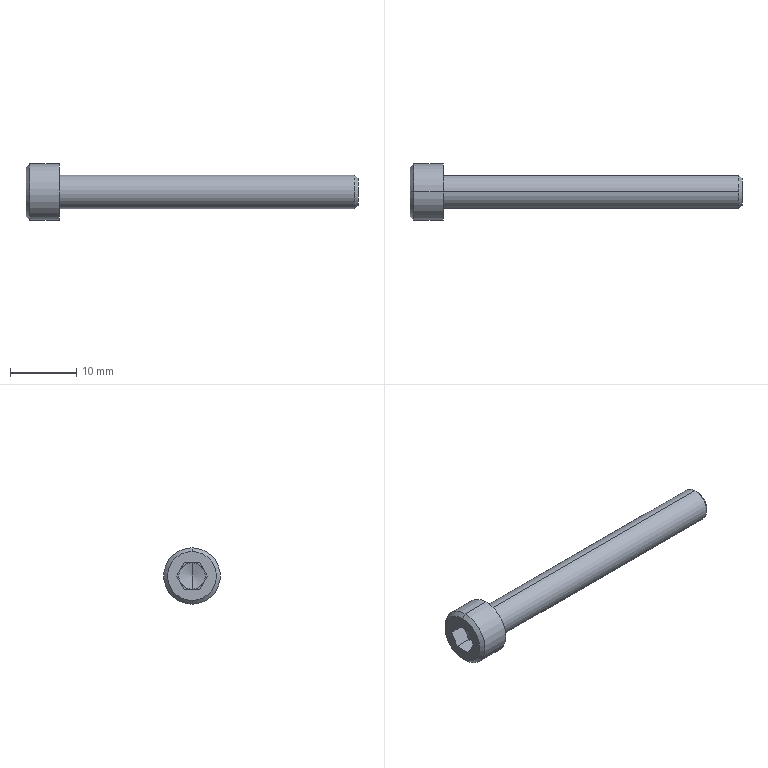Part | SolidWorks | features ICE 1, RevCut 1, Revolution 1 | 1 solid | 25 faces | box 50 x 8.5 x 8.5 mm | volume 1125 mm3 | plane 15 | cone 6 | cylinder 4 | commonest cylinder face diameters 5 x2 8.5 x2